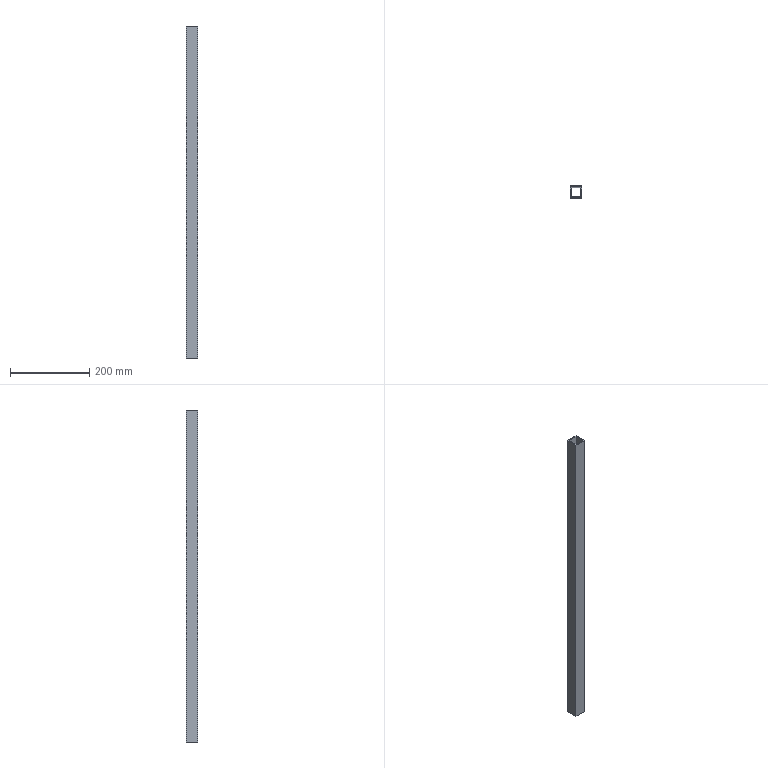Part | SolidWorks | features Extrusion 1, ICE 1 | 1 solid | 10 faces | box 30 x 30 x 840 mm | volume 272160 mm3 | plane 10
STEP:
#1=CARTESIAN_POINT('',(-11.133,32.344,0.));
#2=VERTEX_POINT('',#1);
#3=CARTESIAN_POINT('',(-11.133,2.344,0.));
#4=VERTEX_POINT('',#3);
#5=CARTESIAN_POINT('',(-11.133,2.344,0.));
#6=DIRECTION('',(0.,-1.,0.));
#7=VECTOR('',#6,1000.);
#8=LINE('',#5,#7);
#9=EDGE_CURVE('',#2,#4,#8,.T.);
#10=ORIENTED_EDGE('',*,*,#9,.T.);
#11=CARTESIAN_POINT('',(-11.133,2.344,840.));
#12=VERTEX_POINT('',#11);
#13=CARTESIAN_POINT('',(-11.133,2.344,840.));
#14=DIRECTION('',(0.,0.,-1.));
#15=VECTOR('',#14,1000.);
#16=LINE('',#13,#15);
#17=EDGE_CURVE('',#12,#4,#16,.T.);
#18=ORIENTED_EDGE('',*,*,#17,.F.);
#19=CARTESIAN_POINT('',(-11.133,32.344,840.));
#20=VERTEX_POINT('',#19);
#21=CARTESIAN_POINT('',(-11.133,2.344,840.));
#22=DIRECTION('',(0.,-1.,0.));
#23=VECTOR('',#22,1000.);
#24=LINE('',#21,#23);
#25=EDGE_CURVE('',#20,#12,#24,.T.);
#26=ORIENTED_EDGE('',*,*,#25,.F.);
#27=CARTESIAN_POINT('',(-11.133,32.344,840.));
#28=DIRECTION('',(0.,0.,-1.));
#29=VECTOR('',#28,1000.);
#30=LINE('',#27,#29);
#31=EDGE_CURVE('',#20,#2,#30,.T.);
#32=ORIENTED_EDGE('',*,*,#31,.T.);
#33=EDGE_LOOP('',(#10,#18,#26,#32));
#34=FACE_OUTER_BOUND('',#33,.T.);
#35=CARTESIAN_POINT('',(-11.133,2.344,840.));
#36=DIRECTION('',(1.,0.,0.));
#37=DIRECTION('',(0.,0.,-1.));
#38=AXIS2_PLACEMENT_3D('',#35,#36,#37);
#39=PLANE('',#38);
#40=ADVANCED_FACE('',(#34),#39,.F.);
#41=CARTESIAN_POINT('',(18.867,2.344,0.));
#42=VERTEX_POINT('',#41);
#43=CARTESIAN_POINT('',(18.867,2.344,0.));
#44=DIRECTION('',(1.,0.,0.));
#45=VECTOR('',#44,1000.);
#46=LINE('',#43,#45);
#47=EDGE_CURVE('',#4,#42,#46,.T.);
#48=ORIENTED_EDGE('',*,*,#47,.T.);
#49=CARTESIAN_POINT('',(18.867,2.344,840.));
#50=VERTEX_POINT('',#49);
#51=CARTESIAN_POINT('',(18.867,2.344,840.));
#52=DIRECTION('',(0.,0.,-1.));
#53=VECTOR('',#52,1000.);
#54=LINE('',#51,#53);
#55=EDGE_CURVE('',#50,#42,#54,.T.);
#56=ORIENTED_EDGE('',*,*,#55,.F.);
#57=CARTESIAN_POINT('',(18.867,2.344,840.));
#58=DIRECTION('',(1.,0.,0.));
#59=VECTOR('',#58,1000.);
#60=LINE('',#57,#59);
#61=EDGE_CURVE('',#12,#50,#60,.T.);
#62=ORIENTED_EDGE('',*,*,#61,.F.);
#63=ORIENTED_EDGE('',*,*,#17,.T.);
#64=EDGE_LOOP('',(#48,#56,#62,#63));
#65=FACE_OUTER_BOUND('',#64,.T.);
#66=CARTESIAN_POINT('',(18.867,2.344,840.));
#67=DIRECTION('',(0.,1.,0.));
#68=DIRECTION('',(-1.,0.,0.));
#69=AXIS2_PLACEMENT_3D('',#66,#67,#68);
#70=PLANE('',#69);
#71=ADVANCED_FACE('',(#65),#70,.F.);
#72=CARTESIAN_POINT('',(18.867,32.344,0.));
#73=VERTEX_POINT('',#72);
#74=CARTESIAN_POINT('',(18.867,32.344,0.));
#75=DIRECTION('',(0.,1.,0.));
#76=VECTOR('',#75,1000.);
#77=LINE('',#74,#76);
#78=EDGE_CURVE('',#42,#73,#77,.T.);
#79=ORIENTED_EDGE('',*,*,#78,.T.);
#80=CARTESIAN_POINT('',(18.867,32.344,840.));
#81=VERTEX_POINT('',#80);
#82=CARTESIAN_POINT('',(18.867,32.344,840.));
#83=DIRECTION('',(0.,0.,-1.));
#84=VECTOR('',#83,1000.);
#85=LINE('',#82,#84);
#86=EDGE_CURVE('',#81,#73,#85,.T.);
#87=ORIENTED_EDGE('',*,*,#86,.F.);
#88=CARTESIAN_POINT('',(18.867,32.344,840.));
#89=DIRECTION('',(0.,1.,0.));
#90=VECTOR('',#89,1000.);
#91=LINE('',#88,#90);
#92=EDGE_CURVE('',#50,#81,#91,.T.);
#93=ORIENTED_EDGE('',*,*,#92,.F.);
#94=ORIENTED_EDGE('',*,*,#55,.T.);
#95=EDGE_LOOP('',(#79,#87,#93,#94));
#96=FACE_OUTER_BOUND('',#95,.T.);
#97=CARTESIAN_POINT('',(18.867,32.344,840.));
#98=DIRECTION('',(-1.,0.,0.));
#99=DIRECTION('',(0.,0.,1.));
#100=AXIS2_PLACEMENT_3D('',#97,#98,#99);
#101=PLANE('',#100);
#102=ADVANCED_FACE('',(#96),#101,.F.);
#103=CARTESIAN_POINT('',(-11.133,32.344,0.));
#104=DIRECTION('',(-1.,0.,0.));
#105=VECTOR('',#104,1000.);
#106=LINE('',#103,#105);
#107=EDGE_CURVE('',#73,#2,#106,.T.);
#108=ORIENTED_EDGE('',*,*,#107,.T.);
#109=ORIENTED_EDGE('',*,*,#31,.F.);
#110=CARTESIAN_POINT('',(-11.133,32.344,840.));
#111=DIRECTION('',(-1.,0.,0.));
#112=VECTOR('',#111,1000.);
#113=LINE('',#110,#112);
#114=EDGE_CURVE('',#81,#20,#113,.T.);
#115=ORIENTED_EDGE('',*,*,#114,.F.);
#116=ORIENTED_EDGE('',*,*,#86,.T.);
#117=EDGE_LOOP('',(#108,#109,#115,#116));
#118=FACE_OUTER_BOUND('',#117,.T.);
#119=CARTESIAN_POINT('',(-11.133,32.344,840.));
#120=DIRECTION('',(0.,-1.,0.));
#121=DIRECTION('',(0.,0.,-1.));
#122=AXIS2_PLACEMENT_3D('',#119,#120,#121);
#123=PLANE('',#122);
#124=ADVANCED_FACE('',(#118),#123,.F.);
#125=CARTESIAN_POINT('',(-8.133,5.344,840.));
#126=VERTEX_POINT('',#125);
#127=CARTESIAN_POINT('',(15.867,5.344,840.));
#128=VERTEX_POINT('',#127);
#129=CARTESIAN_POINT('',(15.867,5.344,840.));
#130=DIRECTION('',(1.,0.,0.));
#131=VECTOR('',#130,1000.);
#132=LINE('',#129,#131);
#133=EDGE_CURVE('',#126,#128,#132,.T.);
#134=ORIENTED_EDGE('',*,*,#133,.F.);
#135=CARTESIAN_POINT('',(-8.133,29.344,840.));
#136=VERTEX_POINT('',#135);
#137=CARTESIAN_POINT('',(-8.133,5.344,840.));
#138=DIRECTION('',(0.,-1.,0.));
#139=VECTOR('',#138,1000.);
#140=LINE('',#137,#139);
#141=EDGE_CURVE('',#136,#126,#140,.T.);
#142=ORIENTED_EDGE('',*,*,#141,.F.);
#143=CARTESIAN_POINT('',(15.867,29.344,840.));
#144=VERTEX_POINT('',#143);
#145=CARTESIAN_POINT('',(-8.133,29.344,840.));
#146=DIRECTION('',(-1.,0.,0.));
#147=VECTOR('',#146,1000.);
#148=LINE('',#145,#147);
#149=EDGE_CURVE('',#144,#136,#148,.T.);
#150=ORIENTED_EDGE('',*,*,#149,.F.);
#151=CARTESIAN_POINT('',(15.867,29.344,840.));
#152=DIRECTION('',(0.,1.,0.));
#153=VECTOR('',#152,1000.);
#154=LINE('',#151,#153);
#155=EDGE_CURVE('',#128,#144,#154,.T.);
#156=ORIENTED_EDGE('',*,*,#155,.F.);
#157=EDGE_LOOP('',(#134,#142,#150,#156));
#158=FACE_BOUND('',#157,.T.);
#159=ORIENTED_EDGE('',*,*,#25,.T.);
#160=ORIENTED_EDGE('',*,*,#61,.T.);
#161=ORIENTED_EDGE('',*,*,#92,.T.);
#162=ORIENTED_EDGE('',*,*,#114,.T.);
#163=EDGE_LOOP('',(#159,#160,#161,#162));
#164=FACE_OUTER_BOUND('',#163,.T.);
#165=CARTESIAN_POINT('',(0.,0.,840.));
#166=DIRECTION('',(0.,0.,-1.));
#167=DIRECTION('',(-1.,0.,0.));
#168=AXIS2_PLACEMENT_3D('',#165,#166,#167);
#169=PLANE('',#168);
#170=ADVANCED_FACE('',(#158,#164),#169,.F.);
#171=CARTESIAN_POINT('',(-8.133,29.344,0.));
#172=VERTEX_POINT('',#171);
#173=CARTESIAN_POINT('',(-8.133,5.344,0.));
#174=VERTEX_POINT('',#173);
#175=CARTESIAN_POINT('',(-8.133,5.344,0.));
#176=DIRECTION('',(0.,-1.,0.));
#177=VECTOR('',#176,1000.);
#178=LINE('',#175,#177);
#179=EDGE_CURVE('',#172,#174,#178,.T.);
#180=ORIENTED_EDGE('',*,*,#179,.T.);
#181=CARTESIAN_POINT('',(15.867,5.344,0.));
#182=VERTEX_POINT('',#181);
#183=CARTESIAN_POINT('',(15.867,5.344,0.));
#184=DIRECTION('',(1.,0.,0.));
#185=VECTOR('',#184,1000.);
#186=LINE('',#183,#185);
#187=EDGE_CURVE('',#174,#182,#186,.T.);
#188=ORIENTED_EDGE('',*,*,#187,.T.);
#189=CARTESIAN_POINT('',(15.867,29.344,0.));
#190=VERTEX_POINT('',#189);
#191=CARTESIAN_POINT('',(15.867,29.344,0.));
#192=DIRECTION('',(0.,1.,0.));
#193=VECTOR('',#192,1000.);
#194=LINE('',#191,#193);
#195=EDGE_CURVE('',#182,#190,#194,.T.);
#196=ORIENTED_EDGE('',*,*,#195,.T.);
#197=CARTESIAN_POINT('',(-8.133,29.344,0.));
#198=DIRECTION('',(-1.,0.,0.));
#199=VECTOR('',#198,1000.);
#200=LINE('',#197,#199);
#201=EDGE_CURVE('',#190,#172,#200,.T.);
#202=ORIENTED_EDGE('',*,*,#201,.T.);
#203=EDGE_LOOP('',(#180,#188,#196,#202));
#204=FACE_BOUND('',#203,.T.);
#205=ORIENTED_EDGE('',*,*,#9,.F.);
#206=ORIENTED_EDGE('',*,*,#107,.F.);
#207=ORIENTED_EDGE('',*,*,#78,.F.);
#208=ORIENTED_EDGE('',*,*,#47,.F.);
#209=EDGE_LOOP('',(#205,#206,#207,#208));
#210=FACE_OUTER_BOUND('',#209,.T.);
#211=CARTESIAN_POINT('',(0.,0.,0.));
#212=DIRECTION('',(0.,0.,-1.));
#213=DIRECTION('',(-1.,0.,0.));
#214=AXIS2_PLACEMENT_3D('',#211,#212,#213);
#215=PLANE('',#214);
#216=ADVANCED_FACE('',(#204,#210),#215,.T.);
#217=ORIENTED_EDGE('',*,*,#141,.T.);
#218=CARTESIAN_POINT('',(-8.133,5.344,0.));
#219=DIRECTION('',(0.,0.,1.));
#220=VECTOR('',#219,1000.);
#221=LINE('',#218,#220);
#222=EDGE_CURVE('',#174,#126,#221,.T.);
#223=ORIENTED_EDGE('',*,*,#222,.F.);
#224=ORIENTED_EDGE('',*,*,#179,.F.);
#225=CARTESIAN_POINT('',(-8.133,29.344,0.));
#226=DIRECTION('',(0.,0.,1.));
#227=VECTOR('',#226,1000.);
#228=LINE('',#225,#227);
#229=EDGE_CURVE('',#172,#136,#228,.T.);
#230=ORIENTED_EDGE('',*,*,#229,.T.);
#231=EDGE_LOOP('',(#217,#223,#224,#230));
#232=FACE_OUTER_BOUND('',#231,.T.);
#233=CARTESIAN_POINT('',(-8.133,5.344,0.));
#234=DIRECTION('',(-1.,0.,0.));
#235=DIRECTION('',(0.,0.,1.));
#236=AXIS2_PLACEMENT_3D('',#233,#234,#235);
#237=PLANE('',#236);
#238=ADVANCED_FACE('',(#232),#237,.F.);
#239=ORIENTED_EDGE('',*,*,#149,.T.);
#240=ORIENTED_EDGE('',*,*,#229,.F.);
#241=ORIENTED_EDGE('',*,*,#201,.F.);
#242=CARTESIAN_POINT('',(15.867,29.344,0.));
#243=DIRECTION('',(0.,0.,1.));
#244=VECTOR('',#243,1000.);
#245=LINE('',#242,#244);
#246=EDGE_CURVE('',#190,#144,#245,.T.);
#247=ORIENTED_EDGE('',*,*,#246,.T.);
#248=EDGE_LOOP('',(#239,#240,#241,#247));
#249=FACE_OUTER_BOUND('',#248,.T.);
#250=CARTESIAN_POINT('',(-8.133,29.344,0.));
#251=DIRECTION('',(0.,1.,0.));
#252=DIRECTION('',(0.,0.,1.));
#253=AXIS2_PLACEMENT_3D('',#250,#251,#252);
#254=PLANE('',#253);
#255=ADVANCED_FACE('',(#249),#254,.F.);
#256=ORIENTED_EDGE('',*,*,#155,.T.);
#257=ORIENTED_EDGE('',*,*,#246,.F.);
#258=ORIENTED_EDGE('',*,*,#195,.F.);
#259=CARTESIAN_POINT('',(15.867,5.344,0.));
#260=DIRECTION('',(0.,0.,1.));
#261=VECTOR('',#260,1000.);
#262=LINE('',#259,#261);
#263=EDGE_CURVE('',#182,#128,#262,.T.);
#264=ORIENTED_EDGE('',*,*,#263,.T.);
#265=EDGE_LOOP('',(#256,#257,#258,#264));
#266=FACE_OUTER_BOUND('',#265,.T.);
#267=CARTESIAN_POINT('',(15.867,29.344,0.));
#268=DIRECTION('',(1.,0.,0.));
#269=DIRECTION('',(0.,1.,0.));
#270=AXIS2_PLACEMENT_3D('',#267,#268,#269);
#271=PLANE('',#270);
#272=ADVANCED_FACE('',(#266),#271,.F.);
#273=ORIENTED_EDGE('',*,*,#133,.T.);
#274=ORIENTED_EDGE('',*,*,#263,.F.);
#275=ORIENTED_EDGE('',*,*,#187,.F.);
#276=ORIENTED_EDGE('',*,*,#222,.T.);
#277=EDGE_LOOP('',(#273,#274,#275,#276));
#278=FACE_OUTER_BOUND('',#277,.T.);
#279=CARTESIAN_POINT('',(15.867,5.344,0.));
#280=DIRECTION('',(0.,-1.,0.));
#281=DIRECTION('',(1.,0.,0.));
#282=AXIS2_PLACEMENT_3D('',#279,#280,#281);
#283=PLANE('',#282);
#284=ADVANCED_FACE('',(#278),#283,.F.);
#285=CLOSED_SHELL('',(#40,#71,#102,#124,#170,#216,#238,#255,#272,#284));
#286=MANIFOLD_SOLID_BREP('',#285);
#287=CARTESIAN_POINT('',(0.,0.,0.));
#288=DIRECTION('',(0.,0.,1.));
#289=DIRECTION('',(1.,0.,0.));
#290=AXIS2_PLACEMENT_3D('',#287,#288,#289);
#291=(LENGTH_UNIT()NAMED_UNIT(*)SI_UNIT(.MILLI.,.METRE.));
#292=UNCERTAINTY_MEASURE_WITH_UNIT(LENGTH_MEASURE(0.00001),#291,'','');
#293=(NAMED_UNIT(*)PLANE_ANGLE_UNIT()SI_UNIT($,.RADIAN.));
#294=(NAMED_UNIT(*)SI_UNIT($,.STERADIAN.)SOLID_ANGLE_UNIT());
#295=(GEOMETRIC_REPRESENTATION_CONTEXT(3)GLOBAL_UNCERTAINTY_ASSIGNED_CONTEXT((#292))GLOBAL_UNIT_ASSIGNED_CONTEXT((#291,#293,#294))REPRESENTATION_CONTEXT('',''));
#296=ADVANCED_BREP_SHAPE_REPRESENTATION('',(#286,#290),#295);